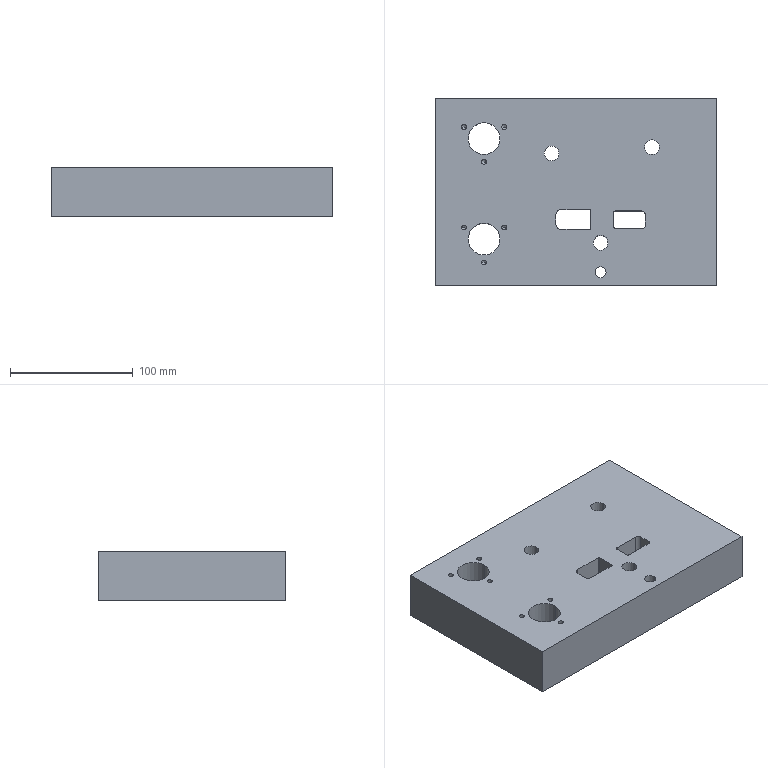Part | 1 solid | 83 faces | box 230 x 153 x 40 mm | volume 1236242 mm3 | cylinder 44 | cone 20 | plane 19 | commonest cylinder face diameters 4 x12 8 x10 12 x10 26 x4 3 x3 1 x2